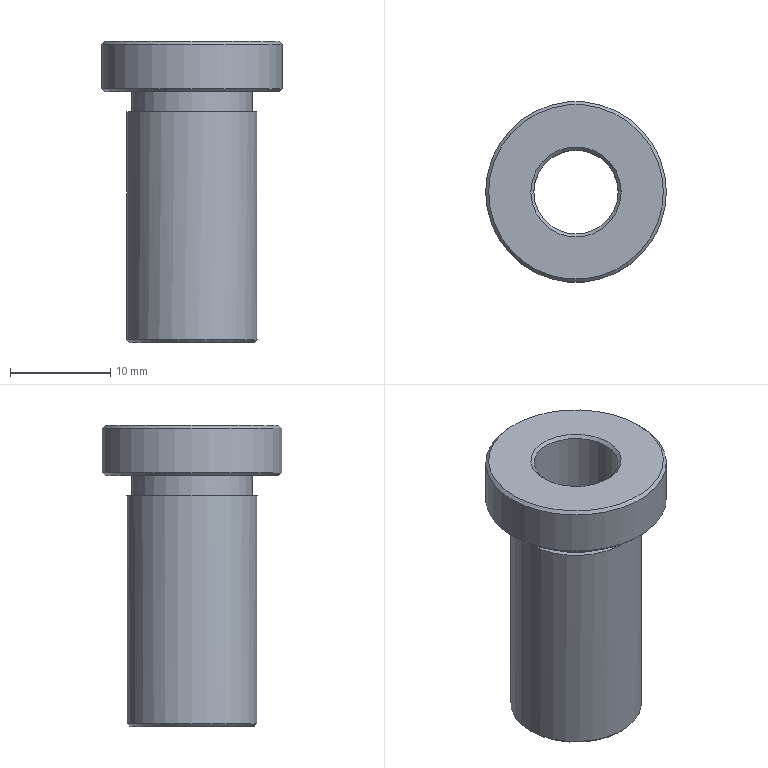Part | STEP file | 200 mesh_id138_x | 1 solid | 13 faces | box 18 x 18 x 30 mm | volume 2880 mm3 | cone 5 | cylinder 4 | plane 4 | commonest cylinder face diameters 8.4 x1 12 x1 13 x1 18 x1
STEP:
#1=CARTESIAN_POINT('',(-16961.384,-4110.269,87.558));
#2=VERTEX_POINT('',#1);
#3=CARTESIAN_POINT('',(-16967.884,-4110.269,87.558));
#4=DIRECTION('',(0.,0.,1.));
#5=DIRECTION('',(1.,0.,0.));
#6=AXIS2_PLACEMENT_3D('',#3,#4,#5);
#7=CIRCLE('',#6,6.5);
#8=EDGE_CURVE('',#2,#2,#7,.T.);
#9=ORIENTED_EDGE('',*,*,#8,.T.);
#10=EDGE_LOOP('',(#9));
#11=FACE_BOUND('',#10,.T.);
#12=CARTESIAN_POINT('',(-16974.384,-4110.269,110.258));
#13=VERTEX_POINT('',#12);
#14=CARTESIAN_POINT('',(-16967.884,-4110.269,110.258));
#15=DIRECTION('',(0.,0.,1.));
#16=DIRECTION('',(-1.,0.,0.));
#17=AXIS2_PLACEMENT_3D('',#14,#15,#16);
#18=CIRCLE('',#17,6.5);
#19=EDGE_CURVE('',#13,#13,#18,.T.);
#20=ORIENTED_EDGE('',*,*,#19,.F.);
#21=EDGE_LOOP('',(#20));
#22=FACE_BOUND('',#21,.T.);
#23=CARTESIAN_POINT('',(-16967.884,-4110.269,112.258));
#24=DIRECTION('',(0.,0.,-1.));
#25=DIRECTION('',(-1.,0.,0.));
#26=AXIS2_PLACEMENT_3D('',#23,#24,#25);
#27=CYLINDRICAL_SURFACE('',#26,6.5);
#28=ADVANCED_FACE('',(#11,#22),#27,.T.);
#29=CARTESIAN_POINT('',(-16972.084,-4110.269,87.558));
#30=VERTEX_POINT('',#29);
#31=CARTESIAN_POINT('',(-16967.884,-4110.269,87.558));
#32=DIRECTION('',(0.,0.,-1.));
#33=DIRECTION('',(-1.,0.,0.));
#34=AXIS2_PLACEMENT_3D('',#31,#32,#33);
#35=CIRCLE('',#34,4.2);
#36=EDGE_CURVE('',#30,#30,#35,.T.);
#37=ORIENTED_EDGE('',*,*,#36,.T.);
#38=EDGE_LOOP('',(#37));
#39=FACE_BOUND('',#38,.T.);
#40=CARTESIAN_POINT('',(-16972.084,-4110.269,116.958));
#41=VERTEX_POINT('',#40);
#42=CARTESIAN_POINT('',(-16967.884,-4110.269,116.958));
#43=DIRECTION('',(0.,0.,1.));
#44=DIRECTION('',(-1.,0.,0.));
#45=AXIS2_PLACEMENT_3D('',#42,#43,#44);
#46=CIRCLE('',#45,4.2);
#47=EDGE_CURVE('',#41,#41,#46,.T.);
#48=ORIENTED_EDGE('',*,*,#47,.T.);
#49=EDGE_LOOP('',(#48));
#50=FACE_BOUND('',#49,.T.);
#51=CARTESIAN_POINT('',(-16967.884,-4110.269,112.258));
#52=DIRECTION('',(0.,0.,-1.));
#53=DIRECTION('',(-1.,0.,0.));
#54=AXIS2_PLACEMENT_3D('',#51,#52,#53);
#55=CYLINDRICAL_SURFACE('',#54,4.2);
#56=ADVANCED_FACE('',(#39,#50),#55,.F.);
#57=CARTESIAN_POINT('',(-16972.384,-4110.269,117.258));
#58=VERTEX_POINT('',#57);
#59=CARTESIAN_POINT('',(-16967.884,-4110.269,117.258));
#60=DIRECTION('',(0.,0.,-1.));
#61=DIRECTION('',(-1.,0.,0.));
#62=AXIS2_PLACEMENT_3D('',#59,#60,#61);
#63=CIRCLE('',#62,4.5);
#64=EDGE_CURVE('',#58,#58,#63,.T.);
#65=ORIENTED_EDGE('',*,*,#64,.T.);
#66=EDGE_LOOP('',(#65));
#67=FACE_BOUND('',#66,.T.);
#68=CARTESIAN_POINT('',(-16976.584,-4110.269,117.258));
#69=VERTEX_POINT('',#68);
#70=CARTESIAN_POINT('',(-16967.884,-4110.269,117.258));
#71=DIRECTION('',(0.,0.,1.));
#72=DIRECTION('',(-1.,0.,0.));
#73=AXIS2_PLACEMENT_3D('',#70,#71,#72);
#74=CIRCLE('',#73,8.7);
#75=EDGE_CURVE('',#69,#69,#74,.T.);
#76=ORIENTED_EDGE('',*,*,#75,.T.);
#77=EDGE_LOOP('',(#76));
#78=FACE_BOUND('',#77,.T.);
#79=CARTESIAN_POINT('',(-16963.684,-4110.269,117.258));
#80=DIRECTION('',(0.,0.,-1.));
#81=DIRECTION('',(-1.,0.,0.));
#82=AXIS2_PLACEMENT_3D('',#79,#80,#81);
#83=PLANE('',#82);
#84=ADVANCED_FACE('',(#67,#78),#83,.F.);
#85=CARTESIAN_POINT('',(-16958.884,-4110.269,112.558));
#86=VERTEX_POINT('',#85);
#87=CARTESIAN_POINT('',(-16967.884,-4110.269,112.558));
#88=DIRECTION('',(0.,0.,1.));
#89=DIRECTION('',(1.,0.,0.));
#90=AXIS2_PLACEMENT_3D('',#87,#88,#89);
#91=CIRCLE('',#90,9.);
#92=EDGE_CURVE('',#86,#86,#91,.T.);
#93=ORIENTED_EDGE('',*,*,#92,.T.);
#94=EDGE_LOOP('',(#93));
#95=FACE_BOUND('',#94,.T.);
#96=CARTESIAN_POINT('',(-16976.884,-4110.269,116.958));
#97=VERTEX_POINT('',#96);
#98=CARTESIAN_POINT('',(-16967.884,-4110.269,116.958));
#99=DIRECTION('',(0.,0.,-1.));
#100=DIRECTION('',(-1.,0.,0.));
#101=AXIS2_PLACEMENT_3D('',#98,#99,#100);
#102=CIRCLE('',#101,9.);
#103=EDGE_CURVE('',#97,#97,#102,.T.);
#104=ORIENTED_EDGE('',*,*,#103,.T.);
#105=EDGE_LOOP('',(#104));
#106=FACE_BOUND('',#105,.T.);
#107=CARTESIAN_POINT('',(-16967.884,-4110.269,112.258));
#108=DIRECTION('',(0.,0.,-1.));
#109=DIRECTION('',(-1.,0.,0.));
#110=AXIS2_PLACEMENT_3D('',#107,#108,#109);
#111=CYLINDRICAL_SURFACE('',#110,9.);
#112=ADVANCED_FACE('',(#95,#106),#111,.T.);
#113=CARTESIAN_POINT('',(-16959.184,-4110.269,112.258));
#114=VERTEX_POINT('',#113);
#115=CARTESIAN_POINT('',(-16967.884,-4110.269,112.258));
#116=DIRECTION('',(0.,0.,-1.));
#117=DIRECTION('',(1.,0.,0.));
#118=AXIS2_PLACEMENT_3D('',#115,#116,#117);
#119=CIRCLE('',#118,8.7);
#120=EDGE_CURVE('',#114,#114,#119,.T.);
#121=ORIENTED_EDGE('',*,*,#120,.T.);
#122=EDGE_LOOP('',(#121));
#123=FACE_BOUND('',#122,.T.);
#124=CARTESIAN_POINT('',(-16961.884,-4110.269,112.258));
#125=VERTEX_POINT('',#124);
#126=CARTESIAN_POINT('',(-16967.884,-4110.269,112.258));
#127=DIRECTION('',(0.,0.,1.));
#128=DIRECTION('',(1.,0.,0.));
#129=AXIS2_PLACEMENT_3D('',#126,#127,#128);
#130=CIRCLE('',#129,6.);
#131=EDGE_CURVE('',#125,#125,#130,.T.);
#132=ORIENTED_EDGE('',*,*,#131,.T.);
#133=EDGE_LOOP('',(#132));
#134=FACE_BOUND('',#133,.T.);
#135=CARTESIAN_POINT('',(-16958.884,-4110.269,112.258));
#136=DIRECTION('',(0.,0.,1.));
#137=DIRECTION('',(1.,0.,0.));
#138=AXIS2_PLACEMENT_3D('',#135,#136,#137);
#139=PLANE('',#138);
#140=ADVANCED_FACE('',(#123,#134),#139,.F.);
#141=CARTESIAN_POINT('',(-16963.384,-4110.269,87.258));
#142=VERTEX_POINT('',#141);
#143=CARTESIAN_POINT('',(-16967.884,-4110.269,87.258));
#144=DIRECTION('',(0.,0.,1.));
#145=DIRECTION('',(1.,0.,0.));
#146=AXIS2_PLACEMENT_3D('',#143,#144,#145);
#147=CIRCLE('',#146,4.5);
#148=EDGE_CURVE('',#142,#142,#147,.T.);
#149=ORIENTED_EDGE('',*,*,#148,.T.);
#150=EDGE_LOOP('',(#149));
#151=FACE_BOUND('',#150,.T.);
#152=CARTESIAN_POINT('',(-16961.684,-4110.269,87.258));
#153=VERTEX_POINT('',#152);
#154=CARTESIAN_POINT('',(-16967.884,-4110.269,87.258));
#155=DIRECTION('',(0.,0.,-1.));
#156=DIRECTION('',(1.,0.,0.));
#157=AXIS2_PLACEMENT_3D('',#154,#155,#156);
#158=CIRCLE('',#157,6.2);
#159=EDGE_CURVE('',#153,#153,#158,.T.);
#160=ORIENTED_EDGE('',*,*,#159,.T.);
#161=EDGE_LOOP('',(#160));
#162=FACE_BOUND('',#161,.T.);
#163=CARTESIAN_POINT('',(-16961.384,-4110.269,87.258));
#164=DIRECTION('',(0.,0.,1.));
#165=DIRECTION('',(1.,0.,0.));
#166=AXIS2_PLACEMENT_3D('',#163,#164,#165);
#167=PLANE('',#166);
#168=ADVANCED_FACE('',(#151,#162),#167,.F.);
#169=ORIENTED_EDGE('',*,*,#36,.F.);
#170=EDGE_LOOP('',(#169));
#171=FACE_BOUND('',#170,.T.);
#172=ORIENTED_EDGE('',*,*,#148,.F.);
#173=EDGE_LOOP('',(#172));
#174=FACE_BOUND('',#173,.T.);
#175=CARTESIAN_POINT('',(-16967.884,-4110.269,87.558));
#176=DIRECTION('',(0.,0.,-1.));
#177=DIRECTION('',(-1.,0.,0.));
#178=AXIS2_PLACEMENT_3D('',#175,#176,#177);
#179=CONICAL_SURFACE('',#178,4.2,45.);
#180=ADVANCED_FACE('',(#171,#174),#179,.F.);
#181=ORIENTED_EDGE('',*,*,#8,.F.);
#182=EDGE_LOOP('',(#181));
#183=FACE_BOUND('',#182,.T.);
#184=ORIENTED_EDGE('',*,*,#159,.F.);
#185=EDGE_LOOP('',(#184));
#186=FACE_BOUND('',#185,.T.);
#187=CARTESIAN_POINT('',(-16967.884,-4110.269,87.258));
#188=DIRECTION('',(0.,0.,1.));
#189=DIRECTION('',(1.,0.,0.));
#190=AXIS2_PLACEMENT_3D('',#187,#188,#189);
#191=CONICAL_SURFACE('',#190,6.2,45.);
#192=ADVANCED_FACE('',(#183,#186),#191,.T.);
#193=CARTESIAN_POINT('',(-16961.884,-4110.269,110.258));
#194=VERTEX_POINT('',#193);
#195=CARTESIAN_POINT('',(-16967.884,-4110.269,110.258));
#196=DIRECTION('',(0.,0.,-1.));
#197=DIRECTION('',(1.,0.,0.));
#198=AXIS2_PLACEMENT_3D('',#195,#196,#197);
#199=CIRCLE('',#198,6.);
#200=EDGE_CURVE('',#194,#194,#199,.T.);
#201=ORIENTED_EDGE('',*,*,#200,.T.);
#202=EDGE_LOOP('',(#201));
#203=FACE_BOUND('',#202,.T.);
#204=ORIENTED_EDGE('',*,*,#19,.T.);
#205=EDGE_LOOP('',(#204));
#206=FACE_BOUND('',#205,.T.);
#207=CARTESIAN_POINT('',(-16967.884,-4110.269,110.258));
#208=DIRECTION('',(0.,0.,-1.));
#209=DIRECTION('',(0.,1.,0.));
#210=AXIS2_PLACEMENT_3D('',#207,#208,#209);
#211=PLANE('',#210);
#212=ADVANCED_FACE('',(#203,#206),#211,.F.);
#213=ORIENTED_EDGE('',*,*,#200,.F.);
#214=EDGE_LOOP('',(#213));
#215=FACE_BOUND('',#214,.T.);
#216=ORIENTED_EDGE('',*,*,#131,.F.);
#217=EDGE_LOOP('',(#216));
#218=FACE_BOUND('',#217,.T.);
#219=CARTESIAN_POINT('',(-16967.884,-4110.269,110.258));
#220=DIRECTION('',(0.,0.,1.));
#221=DIRECTION('',(1.,0.,0.));
#222=AXIS2_PLACEMENT_3D('',#219,#220,#221);
#223=CYLINDRICAL_SURFACE('',#222,6.);
#224=ADVANCED_FACE('',(#215,#218),#223,.T.);
#225=ORIENTED_EDGE('',*,*,#92,.F.);
#226=EDGE_LOOP('',(#225));
#227=FACE_BOUND('',#226,.T.);
#228=ORIENTED_EDGE('',*,*,#120,.F.);
#229=EDGE_LOOP('',(#228));
#230=FACE_BOUND('',#229,.T.);
#231=CARTESIAN_POINT('',(-16967.884,-4110.269,112.258));
#232=DIRECTION('',(0.,0.,1.));
#233=DIRECTION('',(1.,0.,0.));
#234=AXIS2_PLACEMENT_3D('',#231,#232,#233);
#235=CONICAL_SURFACE('',#234,8.7,45.);
#236=ADVANCED_FACE('',(#227,#230),#235,.T.);
#237=ORIENTED_EDGE('',*,*,#75,.F.);
#238=EDGE_LOOP('',(#237));
#239=FACE_BOUND('',#238,.T.);
#240=ORIENTED_EDGE('',*,*,#103,.F.);
#241=EDGE_LOOP('',(#240));
#242=FACE_BOUND('',#241,.T.);
#243=CARTESIAN_POINT('',(-16967.884,-4110.269,116.958));
#244=DIRECTION('',(0.,0.,-1.));
#245=DIRECTION('',(-1.,0.,0.));
#246=AXIS2_PLACEMENT_3D('',#243,#244,#245);
#247=CONICAL_SURFACE('',#246,9.,45.);
#248=ADVANCED_FACE('',(#239,#242),#247,.T.);
#249=ORIENTED_EDGE('',*,*,#47,.F.);
#250=EDGE_LOOP('',(#249));
#251=FACE_BOUND('',#250,.T.);
#252=ORIENTED_EDGE('',*,*,#64,.F.);
#253=EDGE_LOOP('',(#252));
#254=FACE_BOUND('',#253,.T.);
#255=CARTESIAN_POINT('',(-16967.884,-4110.269,117.258));
#256=DIRECTION('',(0.,0.,1.));
#257=DIRECTION('',(1.,0.,0.));
#258=AXIS2_PLACEMENT_3D('',#255,#256,#257);
#259=CONICAL_SURFACE('',#258,4.5,45.);
#260=ADVANCED_FACE('',(#251,#254),#259,.F.);
#261=CLOSED_SHELL('',(#28,#56,#84,#112,#140,#168,#180,#192,#212,#224,#236,#248,#260));
#262=MANIFOLD_SOLID_BREP('',#261);
#263=(LENGTH_UNIT()NAMED_UNIT(*)SI_UNIT(.MILLI.,.METRE.));
#264=UNCERTAINTY_MEASURE_WITH_UNIT(LENGTH_MEASURE(0.00002),#263,'','');
#265=(NAMED_UNIT(*)PLANE_ANGLE_UNIT()SI_UNIT($,.RADIAN.));
#266=PLANE_ANGLE_MEASURE_WITH_UNIT(PLANE_ANGLE_MEASURE(0.01745),#265);
#267=DIMENSIONAL_EXPONENTS(0.,0.,0.,0.,0.,0.,0.);
#268=(CONVERSION_BASED_UNIT('DEGREE',#266)NAMED_UNIT(#267)PLANE_ANGLE_UNIT());
#269=(NAMED_UNIT(*)SI_UNIT($,.STERADIAN.)SOLID_ANGLE_UNIT());
#270=(GEOMETRIC_REPRESENTATION_CONTEXT(3)GLOBAL_UNCERTAINTY_ASSIGNED_CONTEXT((#264))GLOBAL_UNIT_ASSIGNED_CONTEXT((#263,#268,#269))REPRESENTATION_CONTEXT('',''));
#271=ADVANCED_BREP_SHAPE_REPRESENTATION('',(#262),#270);